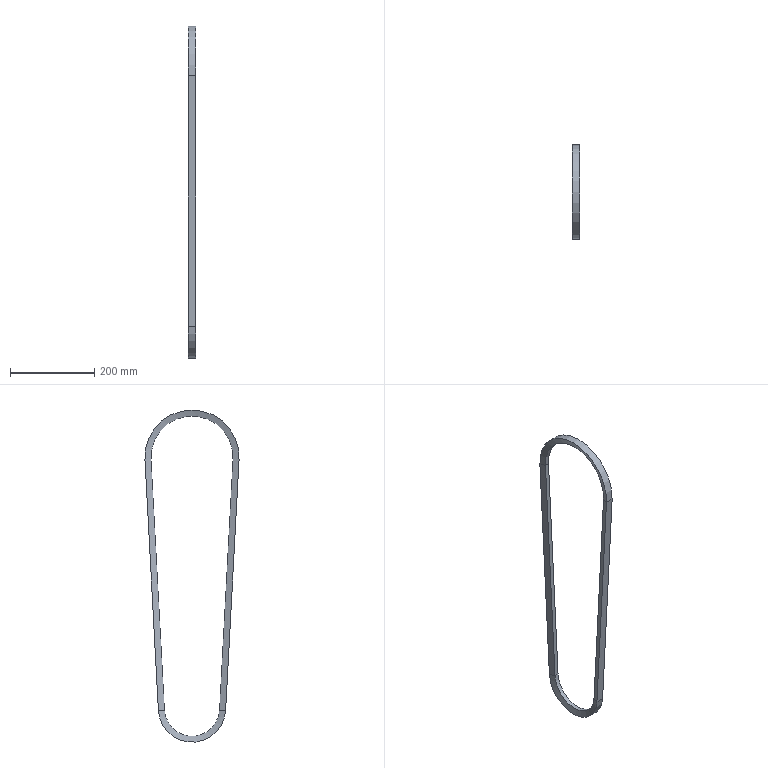Part | NX | features sk_皮带 2 | 1 solid | 16 faces | box 19 x 224 x 789.47 mm | volume 368031 mm3 | plane 8 | cylinder 4 | cone 4 | commonest cylinder face diameters 131.4 x1 160 x1 195.4 x1 224 x1
STEP:
#1=CARTESIAN_POINT('',(-5.128,65.606,-600.989));
#2=VERTEX_POINT('',#1);
#3=CARTESIAN_POINT('',(5.128,65.606,-600.989));
#4=VERTEX_POINT('',#3);
#5=CARTESIAN_POINT('',(5.128,65.606,-600.989));
#6=DIRECTION('',(1.,0.,0.));
#7=VECTOR('',#6,1000.);
#8=LINE('',#5,#7);
#9=EDGE_CURVE('',#2,#4,#8,.T.);
#10=ORIENTED_EDGE('',*,*,#9,.T.);
#11=CARTESIAN_POINT('',(5.128,97.56,-5.233));
#12=VERTEX_POINT('',#11);
#13=CARTESIAN_POINT('',(5.128,65.606,-600.989));
#14=DIRECTION('',(0.,0.05356,0.9986));
#15=VECTOR('',#14,1000.);
#16=LINE('',#13,#15);
#17=EDGE_CURVE('',#4,#12,#16,.T.);
#18=ORIENTED_EDGE('',*,*,#17,.T.);
#19=CARTESIAN_POINT('',(-5.128,97.56,-5.233));
#20=VERTEX_POINT('',#19);
#21=CARTESIAN_POINT('',(5.128,97.56,-5.233));
#22=DIRECTION('',(1.,0.,0.));
#23=VECTOR('',#22,1000.);
#24=LINE('',#21,#23);
#25=EDGE_CURVE('',#20,#12,#24,.T.);
#26=ORIENTED_EDGE('',*,*,#25,.F.);
#27=CARTESIAN_POINT('',(-5.128,65.606,-600.989));
#28=DIRECTION('',(0.,0.05356,0.9986));
#29=VECTOR('',#28,1000.);
#30=LINE('',#27,#29);
#31=EDGE_CURVE('',#2,#20,#30,.T.);
#32=ORIENTED_EDGE('',*,*,#31,.F.);
#33=EDGE_LOOP('',(#10,#18,#26,#32));
#34=FACE_BOUND('',#33,.T.);
#35=CARTESIAN_POINT('',(5.128,65.606,-600.989));
#36=DIRECTION('',(0.,-0.9986,0.05356));
#37=DIRECTION('',(0.,-0.05356,-0.9986));
#38=AXIS2_PLACEMENT_3D('',#35,#36,#37);
#39=PLANE('',#38);
#40=ADVANCED_FACE('',(#34),#39,.T.);
#41=CARTESIAN_POINT('',(9.5,79.885,-601.755));
#42=VERTEX_POINT('',#41);
#43=CARTESIAN_POINT('',(9.5,79.885,-601.755));
#44=DIRECTION('',(0.2924,0.9549,-0.05122));
#45=VECTOR('',#44,1000.);
#46=LINE('',#43,#45);
#47=EDGE_CURVE('',#4,#42,#46,.T.);
#48=ORIENTED_EDGE('',*,*,#47,.T.);
#49=CARTESIAN_POINT('',(9.5,111.839,-5.999));
#50=VERTEX_POINT('',#49);
#51=CARTESIAN_POINT('',(9.5,79.885,-601.755));
#52=DIRECTION('',(0.,0.05356,0.9986));
#53=VECTOR('',#52,1000.);
#54=LINE('',#51,#53);
#55=EDGE_CURVE('',#42,#50,#54,.T.);
#56=ORIENTED_EDGE('',*,*,#55,.T.);
#57=CARTESIAN_POINT('',(9.5,111.839,-5.999));
#58=DIRECTION('',(0.2924,0.9549,-0.05122));
#59=VECTOR('',#58,1000.);
#60=LINE('',#57,#59);
#61=EDGE_CURVE('',#12,#50,#60,.T.);
#62=ORIENTED_EDGE('',*,*,#61,.F.);
#63=ORIENTED_EDGE('',*,*,#17,.F.);
#64=EDGE_LOOP('',(#48,#56,#62,#63));
#65=FACE_BOUND('',#64,.T.);
#66=CARTESIAN_POINT('',(9.5,79.885,-601.755));
#67=DIRECTION('',(0.9563,-0.292,0.01566));
#68=DIRECTION('',(0.292,0.9564,0.));
#69=AXIS2_PLACEMENT_3D('',#66,#67,#68);
#70=PLANE('',#69);
#71=ADVANCED_FACE('',(#65),#70,.T.);
#72=CARTESIAN_POINT('',(-9.5,79.885,-601.755));
#73=VERTEX_POINT('',#72);
#74=CARTESIAN_POINT('',(-9.5,79.885,-601.755));
#75=DIRECTION('',(-1.,0.,0.));
#76=VECTOR('',#75,1000.);
#77=LINE('',#74,#76);
#78=EDGE_CURVE('',#42,#73,#77,.T.);
#79=ORIENTED_EDGE('',*,*,#78,.T.);
#80=CARTESIAN_POINT('',(-9.5,111.839,-5.999));
#81=VERTEX_POINT('',#80);
#82=CARTESIAN_POINT('',(-9.5,79.885,-601.755));
#83=DIRECTION('',(0.,0.05356,0.9986));
#84=VECTOR('',#83,1000.);
#85=LINE('',#82,#84);
#86=EDGE_CURVE('',#73,#81,#85,.T.);
#87=ORIENTED_EDGE('',*,*,#86,.T.);
#88=CARTESIAN_POINT('',(-9.5,111.839,-5.999));
#89=DIRECTION('',(-1.,0.,0.));
#90=VECTOR('',#89,1000.);
#91=LINE('',#88,#90);
#92=EDGE_CURVE('',#50,#81,#91,.T.);
#93=ORIENTED_EDGE('',*,*,#92,.F.);
#94=ORIENTED_EDGE('',*,*,#55,.F.);
#95=EDGE_LOOP('',(#79,#87,#93,#94));
#96=FACE_BOUND('',#95,.T.);
#97=CARTESIAN_POINT('',(-9.5,79.885,-601.755));
#98=DIRECTION('',(0.,0.9986,-0.05356));
#99=DIRECTION('',(0.,0.05356,0.9986));
#100=AXIS2_PLACEMENT_3D('',#97,#98,#99);
#101=PLANE('',#100);
#102=ADVANCED_FACE('',(#96),#101,.T.);
#103=CARTESIAN_POINT('',(-5.128,65.606,-600.989));
#104=DIRECTION('',(0.2924,-0.9549,0.05122));
#105=VECTOR('',#104,1000.);
#106=LINE('',#103,#105);
#107=EDGE_CURVE('',#73,#2,#106,.T.);
#108=ORIENTED_EDGE('',*,*,#107,.T.);
#109=ORIENTED_EDGE('',*,*,#31,.T.);
#110=CARTESIAN_POINT('',(-5.128,97.56,-5.233));
#111=DIRECTION('',(0.2924,-0.9549,0.05122));
#112=VECTOR('',#111,1000.);
#113=LINE('',#110,#112);
#114=EDGE_CURVE('',#81,#20,#113,.T.);
#115=ORIENTED_EDGE('',*,*,#114,.F.);
#116=ORIENTED_EDGE('',*,*,#86,.F.);
#117=EDGE_LOOP('',(#108,#109,#115,#116));
#118=FACE_BOUND('',#117,.T.);
#119=CARTESIAN_POINT('',(-5.128,65.606,-600.989));
#120=DIRECTION('',(-0.9563,-0.292,0.01566));
#121=DIRECTION('',(0.292,-0.9564,0.));
#122=AXIS2_PLACEMENT_3D('',#119,#120,#121);
#123=PLANE('',#122);
#124=ADVANCED_FACE('',(#118),#123,.T.);
#125=CARTESIAN_POINT('',(-5.128,-65.606,-600.989));
#126=VERTEX_POINT('',#125);
#127=CARTESIAN_POINT('',(5.128,-65.606,-600.989));
#128=VERTEX_POINT('',#127);
#129=CARTESIAN_POINT('',(5.128,-65.606,-600.989));
#130=DIRECTION('',(1.,0.,0.));
#131=VECTOR('',#130,1000.);
#132=LINE('',#129,#131);
#133=EDGE_CURVE('',#126,#128,#132,.T.);
#134=ORIENTED_EDGE('',*,*,#133,.T.);
#135=CARTESIAN_POINT('',(5.128,0.,-597.47));
#136=DIRECTION('',(1.,0.,0.));
#137=DIRECTION('',(0.,0.,-1.));
#138=AXIS2_PLACEMENT_3D('',#135,#136,#137);
#139=CIRCLE('',#138,65.7);
#140=EDGE_CURVE('',#128,#4,#139,.T.);
#141=ORIENTED_EDGE('',*,*,#140,.T.);
#142=ORIENTED_EDGE('',*,*,#9,.F.);
#143=CARTESIAN_POINT('',(-5.128,0.,-597.47));
#144=DIRECTION('',(1.,0.,0.));
#145=DIRECTION('',(0.,0.,-1.));
#146=AXIS2_PLACEMENT_3D('',#143,#144,#145);
#147=CIRCLE('',#146,65.7);
#148=EDGE_CURVE('',#126,#2,#147,.T.);
#149=ORIENTED_EDGE('',*,*,#148,.F.);
#150=EDGE_LOOP('',(#134,#141,#142,#149));
#151=FACE_BOUND('',#150,.T.);
#152=CARTESIAN_POINT('',(0.,0.,-597.47));
#153=DIRECTION('',(1.,0.,0.));
#154=DIRECTION('',(0.,0.,-1.));
#155=AXIS2_PLACEMENT_3D('',#152,#153,#154);
#156=CYLINDRICAL_SURFACE('',#155,65.7);
#157=ADVANCED_FACE('',(#151),#156,.F.);
#158=CARTESIAN_POINT('',(9.5,-79.885,-601.755));
#159=VERTEX_POINT('',#158);
#160=CARTESIAN_POINT('',(9.5,-79.885,-601.755));
#161=DIRECTION('',(0.2924,-0.9549,-0.05122));
#162=VECTOR('',#161,1000.);
#163=LINE('',#160,#162);
#164=EDGE_CURVE('',#128,#159,#163,.T.);
#165=ORIENTED_EDGE('',*,*,#164,.T.);
#166=CARTESIAN_POINT('',(9.5,0.,-597.47));
#167=DIRECTION('',(1.,0.,0.));
#168=DIRECTION('',(0.,0.,-1.));
#169=AXIS2_PLACEMENT_3D('',#166,#167,#168);
#170=CIRCLE('',#169,80.);
#171=EDGE_CURVE('',#159,#42,#170,.T.);
#172=ORIENTED_EDGE('',*,*,#171,.T.);
#173=ORIENTED_EDGE('',*,*,#47,.F.);
#174=ORIENTED_EDGE('',*,*,#140,.F.);
#175=EDGE_LOOP('',(#165,#172,#173,#174));
#176=FACE_BOUND('',#175,.T.);
#177=CARTESIAN_POINT('',(5.128,0.,-597.47));
#178=DIRECTION('',(1.,0.,0.));
#179=DIRECTION('',(0.,0.,-1.));
#180=AXIS2_PLACEMENT_3D('',#177,#178,#179);
#181=CONICAL_SURFACE('',#180,65.7,1.274);
#182=ADVANCED_FACE('',(#176),#181,.F.);
#183=CARTESIAN_POINT('',(-9.5,-79.885,-601.755));
#184=VERTEX_POINT('',#183);
#185=CARTESIAN_POINT('',(-9.5,-79.885,-601.755));
#186=DIRECTION('',(-1.,0.,0.));
#187=VECTOR('',#186,1000.);
#188=LINE('',#185,#187);
#189=EDGE_CURVE('',#159,#184,#188,.T.);
#190=ORIENTED_EDGE('',*,*,#189,.T.);
#191=CARTESIAN_POINT('',(-9.5,0.,-597.47));
#192=DIRECTION('',(1.,0.,0.));
#193=DIRECTION('',(0.,0.,-1.));
#194=AXIS2_PLACEMENT_3D('',#191,#192,#193);
#195=CIRCLE('',#194,80.);
#196=EDGE_CURVE('',#184,#73,#195,.T.);
#197=ORIENTED_EDGE('',*,*,#196,.T.);
#198=ORIENTED_EDGE('',*,*,#78,.F.);
#199=ORIENTED_EDGE('',*,*,#171,.F.);
#200=EDGE_LOOP('',(#190,#197,#198,#199));
#201=FACE_BOUND('',#200,.T.);
#202=CARTESIAN_POINT('',(0.,0.,-597.47));
#203=DIRECTION('',(1.,0.,0.));
#204=DIRECTION('',(0.,0.,-1.));
#205=AXIS2_PLACEMENT_3D('',#202,#203,#204);
#206=CYLINDRICAL_SURFACE('',#205,80.);
#207=ADVANCED_FACE('',(#201),#206,.T.);
#208=CARTESIAN_POINT('',(-5.128,-65.606,-600.989));
#209=DIRECTION('',(0.2924,0.9549,0.05122));
#210=VECTOR('',#209,1000.);
#211=LINE('',#208,#210);
#212=EDGE_CURVE('',#184,#126,#211,.T.);
#213=ORIENTED_EDGE('',*,*,#212,.T.);
#214=ORIENTED_EDGE('',*,*,#148,.T.);
#215=ORIENTED_EDGE('',*,*,#107,.F.);
#216=ORIENTED_EDGE('',*,*,#196,.F.);
#217=EDGE_LOOP('',(#213,#214,#215,#216));
#218=FACE_BOUND('',#217,.T.);
#219=CARTESIAN_POINT('',(-9.5,0.,-597.47));
#220=DIRECTION('',(-1.,0.,0.));
#221=DIRECTION('',(0.,0.,1.));
#222=AXIS2_PLACEMENT_3D('',#219,#220,#221);
#223=CONICAL_SURFACE('',#222,80.,1.274);
#224=ADVANCED_FACE('',(#218),#223,.F.);
#225=CARTESIAN_POINT('',(-5.128,-97.56,-5.233));
#226=VERTEX_POINT('',#225);
#227=CARTESIAN_POINT('',(5.128,-97.56,-5.233));
#228=VERTEX_POINT('',#227);
#229=CARTESIAN_POINT('',(5.128,-97.56,-5.233));
#230=DIRECTION('',(1.,0.,0.));
#231=VECTOR('',#230,1000.);
#232=LINE('',#229,#231);
#233=EDGE_CURVE('',#226,#228,#232,.T.);
#234=ORIENTED_EDGE('',*,*,#233,.T.);
#235=CARTESIAN_POINT('',(5.128,-97.56,-5.233));
#236=DIRECTION('',(0.,0.05356,-0.9986));
#237=VECTOR('',#236,1000.);
#238=LINE('',#235,#237);
#239=EDGE_CURVE('',#228,#128,#238,.T.);
#240=ORIENTED_EDGE('',*,*,#239,.T.);
#241=ORIENTED_EDGE('',*,*,#133,.F.);
#242=CARTESIAN_POINT('',(-5.128,-97.56,-5.233));
#243=DIRECTION('',(0.,0.05356,-0.9986));
#244=VECTOR('',#243,1000.);
#245=LINE('',#242,#244);
#246=EDGE_CURVE('',#226,#126,#245,.T.);
#247=ORIENTED_EDGE('',*,*,#246,.F.);
#248=EDGE_LOOP('',(#234,#240,#241,#247));
#249=FACE_BOUND('',#248,.T.);
#250=CARTESIAN_POINT('',(5.128,-97.56,-5.233));
#251=DIRECTION('',(0.,0.9986,0.05356));
#252=DIRECTION('',(0.,-0.05356,0.9986));
#253=AXIS2_PLACEMENT_3D('',#250,#251,#252);
#254=PLANE('',#253);
#255=ADVANCED_FACE('',(#249),#254,.T.);
#256=CARTESIAN_POINT('',(9.5,-111.839,-5.999));
#257=VERTEX_POINT('',#256);
#258=CARTESIAN_POINT('',(9.5,-111.839,-5.999));
#259=DIRECTION('',(0.2924,-0.9549,-0.05122));
#260=VECTOR('',#259,1000.);
#261=LINE('',#258,#260);
#262=EDGE_CURVE('',#228,#257,#261,.T.);
#263=ORIENTED_EDGE('',*,*,#262,.T.);
#264=CARTESIAN_POINT('',(9.5,-111.839,-5.999));
#265=DIRECTION('',(0.,0.05356,-0.9986));
#266=VECTOR('',#265,1000.);
#267=LINE('',#264,#266);
#268=EDGE_CURVE('',#257,#159,#267,.T.);
#269=ORIENTED_EDGE('',*,*,#268,.T.);
#270=ORIENTED_EDGE('',*,*,#164,.F.);
#271=ORIENTED_EDGE('',*,*,#239,.F.);
#272=EDGE_LOOP('',(#263,#269,#270,#271));
#273=FACE_BOUND('',#272,.T.);
#274=CARTESIAN_POINT('',(9.5,-111.839,-5.999));
#275=DIRECTION('',(0.9563,0.292,0.01566));
#276=DIRECTION('',(-0.292,0.9564,0.));
#277=AXIS2_PLACEMENT_3D('',#274,#275,#276);
#278=PLANE('',#277);
#279=ADVANCED_FACE('',(#273),#278,.T.);
#280=CARTESIAN_POINT('',(-9.5,-111.839,-5.999));
#281=VERTEX_POINT('',#280);
#282=CARTESIAN_POINT('',(-9.5,-111.839,-5.999));
#283=DIRECTION('',(-1.,0.,0.));
#284=VECTOR('',#283,1000.);
#285=LINE('',#282,#284);
#286=EDGE_CURVE('',#257,#281,#285,.T.);
#287=ORIENTED_EDGE('',*,*,#286,.T.);
#288=CARTESIAN_POINT('',(-9.5,-111.839,-5.999));
#289=DIRECTION('',(0.,0.05356,-0.9986));
#290=VECTOR('',#289,1000.);
#291=LINE('',#288,#290);
#292=EDGE_CURVE('',#281,#184,#291,.T.);
#293=ORIENTED_EDGE('',*,*,#292,.T.);
#294=ORIENTED_EDGE('',*,*,#189,.F.);
#295=ORIENTED_EDGE('',*,*,#268,.F.);
#296=EDGE_LOOP('',(#287,#293,#294,#295));
#297=FACE_BOUND('',#296,.T.);
#298=CARTESIAN_POINT('',(-9.5,-111.839,-5.999));
#299=DIRECTION('',(0.,-0.9986,-0.05356));
#300=DIRECTION('',(0.,0.05356,-0.9986));
#301=AXIS2_PLACEMENT_3D('',#298,#299,#300);
#302=PLANE('',#301);
#303=ADVANCED_FACE('',(#297),#302,.T.);
#304=CARTESIAN_POINT('',(-5.128,-97.56,-5.233));
#305=DIRECTION('',(0.2924,0.9549,0.05122));
#306=VECTOR('',#305,1000.);
#307=LINE('',#304,#306);
#308=EDGE_CURVE('',#281,#226,#307,.T.);
#309=ORIENTED_EDGE('',*,*,#308,.T.);
#310=ORIENTED_EDGE('',*,*,#246,.T.);
#311=ORIENTED_EDGE('',*,*,#212,.F.);
#312=ORIENTED_EDGE('',*,*,#292,.F.);
#313=EDGE_LOOP('',(#309,#310,#311,#312));
#314=FACE_BOUND('',#313,.T.);
#315=CARTESIAN_POINT('',(-5.128,-97.56,-5.233));
#316=DIRECTION('',(-0.9563,0.292,0.01566));
#317=DIRECTION('',(-0.292,-0.9564,0.));
#318=AXIS2_PLACEMENT_3D('',#315,#316,#317);
#319=PLANE('',#318);
#320=ADVANCED_FACE('',(#314),#319,.T.);
#321=CARTESIAN_POINT('',(-9.5,0.,0.));
#322=DIRECTION('',(-1.,0.,0.));
#323=DIRECTION('',(0.,0.,1.));
#324=AXIS2_PLACEMENT_3D('',#321,#322,#323);
#325=CIRCLE('',#324,112.);
#326=EDGE_CURVE('',#281,#81,#325,.T.);
#327=ORIENTED_EDGE('',*,*,#326,.T.);
#328=ORIENTED_EDGE('',*,*,#114,.T.);
#329=CARTESIAN_POINT('',(-5.128,0.,0.));
#330=DIRECTION('',(-1.,0.,0.));
#331=DIRECTION('',(0.,0.,1.));
#332=AXIS2_PLACEMENT_3D('',#329,#330,#331);
#333=CIRCLE('',#332,97.7);
#334=EDGE_CURVE('',#226,#20,#333,.T.);
#335=ORIENTED_EDGE('',*,*,#334,.F.);
#336=ORIENTED_EDGE('',*,*,#308,.F.);
#337=EDGE_LOOP('',(#327,#328,#335,#336));
#338=FACE_BOUND('',#337,.T.);
#339=CARTESIAN_POINT('',(-9.5,0.,0.));
#340=DIRECTION('',(-1.,0.,0.));
#341=DIRECTION('',(0.,0.,1.));
#342=AXIS2_PLACEMENT_3D('',#339,#340,#341);
#343=CONICAL_SURFACE('',#342,112.,1.274);
#344=ADVANCED_FACE('',(#338),#343,.F.);
#345=CARTESIAN_POINT('',(9.5,0.,0.));
#346=DIRECTION('',(-1.,0.,0.));
#347=DIRECTION('',(0.,0.,1.));
#348=AXIS2_PLACEMENT_3D('',#345,#346,#347);
#349=CIRCLE('',#348,112.);
#350=EDGE_CURVE('',#257,#50,#349,.T.);
#351=ORIENTED_EDGE('',*,*,#350,.T.);
#352=ORIENTED_EDGE('',*,*,#92,.T.);
#353=ORIENTED_EDGE('',*,*,#326,.F.);
#354=ORIENTED_EDGE('',*,*,#286,.F.);
#355=EDGE_LOOP('',(#351,#352,#353,#354));
#356=FACE_BOUND('',#355,.T.);
#357=CARTESIAN_POINT('',(0.,0.,0.));
#358=DIRECTION('',(-1.,0.,0.));
#359=DIRECTION('',(0.,0.,1.));
#360=AXIS2_PLACEMENT_3D('',#357,#358,#359);
#361=CYLINDRICAL_SURFACE('',#360,112.);
#362=ADVANCED_FACE('',(#356),#361,.T.);
#363=CARTESIAN_POINT('',(5.128,0.,0.));
#364=DIRECTION('',(-1.,0.,0.));
#365=DIRECTION('',(0.,0.,1.));
#366=AXIS2_PLACEMENT_3D('',#363,#364,#365);
#367=CIRCLE('',#366,97.7);
#368=EDGE_CURVE('',#228,#12,#367,.T.);
#369=ORIENTED_EDGE('',*,*,#368,.T.);
#370=ORIENTED_EDGE('',*,*,#61,.T.);
#371=ORIENTED_EDGE('',*,*,#350,.F.);
#372=ORIENTED_EDGE('',*,*,#262,.F.);
#373=EDGE_LOOP('',(#369,#370,#371,#372));
#374=FACE_BOUND('',#373,.T.);
#375=CARTESIAN_POINT('',(5.128,0.,0.));
#376=DIRECTION('',(1.,0.,0.));
#377=DIRECTION('',(0.,0.,-1.));
#378=AXIS2_PLACEMENT_3D('',#375,#376,#377);
#379=CONICAL_SURFACE('',#378,97.7,1.274);
#380=ADVANCED_FACE('',(#374),#379,.F.);
#381=ORIENTED_EDGE('',*,*,#233,.F.);
#382=ORIENTED_EDGE('',*,*,#334,.T.);
#383=ORIENTED_EDGE('',*,*,#25,.T.);
#384=ORIENTED_EDGE('',*,*,#368,.F.);
#385=EDGE_LOOP('',(#381,#382,#383,#384));
#386=FACE_BOUND('',#385,.T.);
#387=CARTESIAN_POINT('',(0.,0.,0.));
#388=DIRECTION('',(-1.,0.,0.));
#389=DIRECTION('',(0.,0.,1.));
#390=AXIS2_PLACEMENT_3D('',#387,#388,#389);
#391=CYLINDRICAL_SURFACE('',#390,97.7);
#392=ADVANCED_FACE('',(#386),#391,.F.);
#393=CLOSED_SHELL('',(#40,#71,#102,#124,#157,#182,#207,#224,#255,#279,#303,#320,#344,#362,#380,#392));
#394=MANIFOLD_SOLID_BREP('',#393);
#395=(LENGTH_UNIT()NAMED_UNIT(*)SI_UNIT(.MILLI.,.METRE.));
#396=UNCERTAINTY_MEASURE_WITH_UNIT(LENGTH_MEASURE(0.00001),#395,'','');
#397=(NAMED_UNIT(*)PLANE_ANGLE_UNIT()SI_UNIT($,.RADIAN.));
#398=(NAMED_UNIT(*)SI_UNIT($,.STERADIAN.)SOLID_ANGLE_UNIT());
#399=(GEOMETRIC_REPRESENTATION_CONTEXT(3)GLOBAL_UNCERTAINTY_ASSIGNED_CONTEXT((#396))GLOBAL_UNIT_ASSIGNED_CONTEXT((#395,#397,#398))REPRESENTATION_CONTEXT('',''));
#400=ADVANCED_BREP_SHAPE_REPRESENTATION('',(#394),#399);